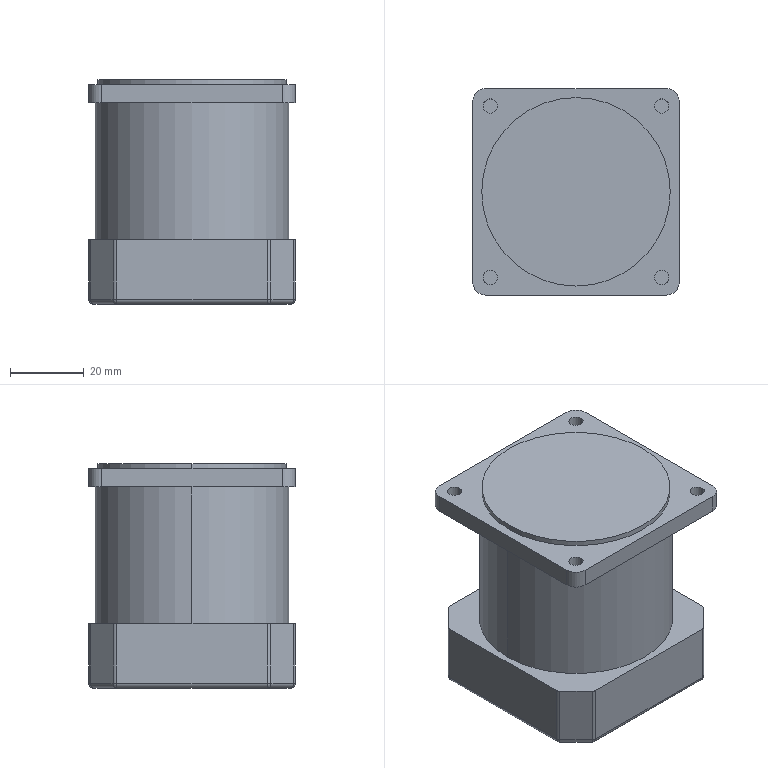Part | SolidWorks | features SplitBody 1 | 1 solid | 57 faces | box 56 x 56 x 60.9 mm | volume 151343 mm3 | cylinder 32 | plane 17 | sphere 8 | commonest cylinder face diameters 2.8 x16 3.85 x8 7 x4 51.1 x2 52.5 x2